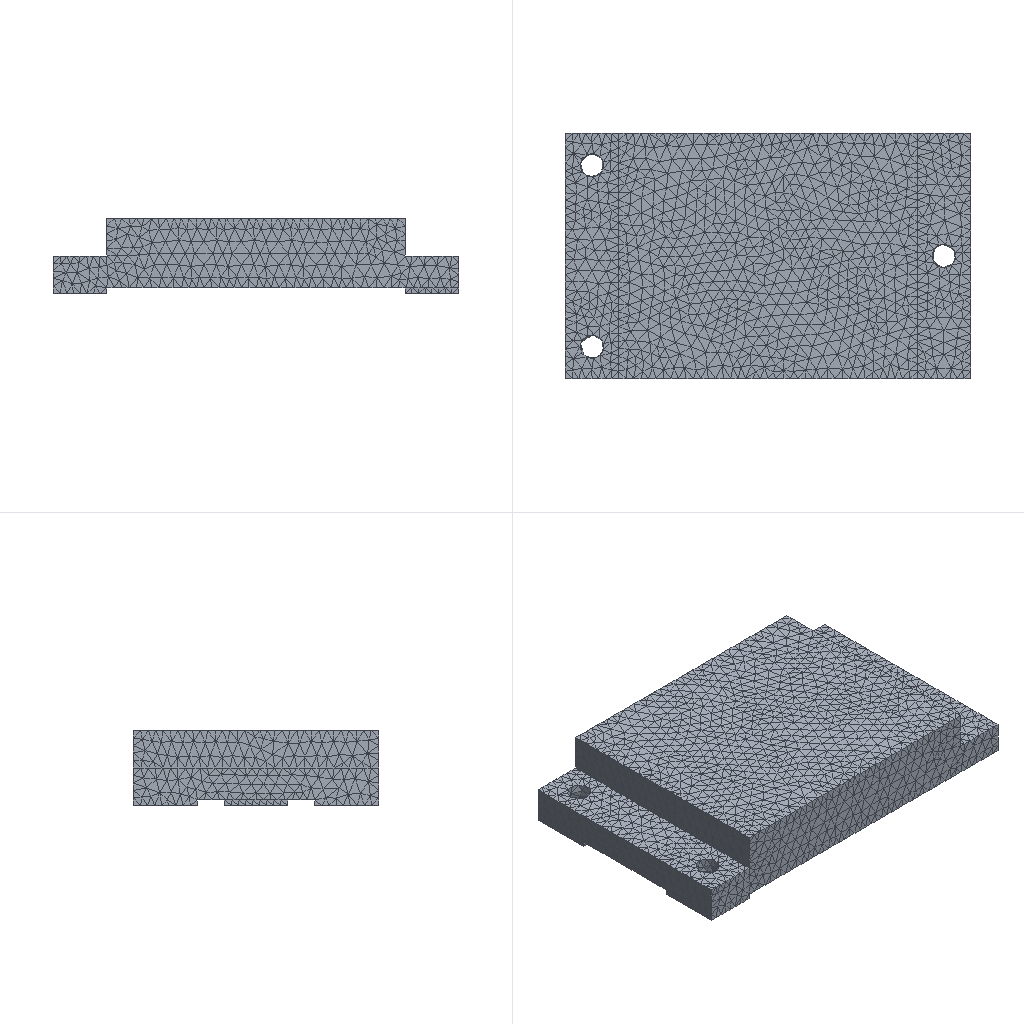Simulation study | ansys workbench
Set-up summary:
category,name,step,type,value,unit,region
solver,ansys_workbench
units,SI m-kg-s (Pa),,stated,"/units,MKS"
analysis,LS1,,static
load_step,LS1,LS1,static,nsubst=1; time=1
mesh,nodes,,,33082
mesh,elements,,,20941
element_type,SOLID187,,,19645
element_type,CONTA174,,,1296
material,Structural Steel,,E,2e+11,Pa
material,Structural Steel,,nu,0.3
material,Structural Steel,,density,7850,kg m^-3
material,Structural Steel,,conductivity,60.5,W m^-1 C^-1
material,Structural Steel,,specific_heat,434,J kg^-1 C^-1
material,Structural Steel,,cte,1.2e-05,C^-1
material,Structural Steel,,permeability,10000
material,Structural Steel,,resistivity,1.7e-07,kg m^3 A^-2 s^-3
load,,LS1,moment,"1500 [dir=(0, 0, 1) n=3]",,all
bc,Fixed Supports,model,fixed,[dofs=ALL],,_FIXEDSU
contact,contact 1,,bonded (always),element=CONTA174
named_set,_FIXEDSU,,node,597
Ansys APDL input file, long lists of numbers shortened:
/batch
/config,noeldb,1     ! force off writing results to database
*get,_wallstrt,active,,time,wall
! ANSYS input file written by Workbench version 2024 R1
! File used for geometry attach:
/title,wbnew--____ (A5)
! ****** Begin Custom Load Command Snippet ******
/COM, ACT Extensions:
/COM,     LSDYNA, 2024.1
/COM,/COM,     ANSYSMotion, 2024.1
/COM,
! ****** End   Custom Load Command Snippet ******
*DIM,_wb_ProjectScratch_dir,string,248
_wb_ProjectScratch_dir(1) = ''
*DIM,_wb_SolverFiles_dir,string,248
_wb_SolverFiles_dir(1) = ''
*DIM,_wb_userfiles_dir,string,248
_wb_userfiles_dir(1) = ''
/com,--- Data in consistent MKS units. See Solving Units in the help system for more information.
/units,MKS
/nopr
/wb,file,start              !  signify a WB generated input file
/prep7
! Turn off shape checking because checks already performed inside WB mesher.
! See help system for more information.
SHPP,OFF,,NOWARN
/nolist
etcon,set             ! allow ANSYS to choose best KEYOP's for 180x elements, resets any applicable keyopt to MAPDL defaults
/com,*********** Nodes for the whole assembly ***********
nblock,3,,36389
(1i9,3e20.9e3)
        1     7.600000000E-02     0.000000000E+00     1.000000000E-03
! (33080 more lines like these left out)
-1
/com,*********** Nodes for all Remote Points ***********
nblock,3
(1i9,3e20.9e3)
    33082     3.800000000E-02     2.300000000E-02     1.400000000E-02
-1
/wb,elem,start            !  set before creation of elements
/com,*********** Elements for Body 1 "__ - Camera Link" ***********
et,1,187
eblock,19,solid,,19645
(19i9)
        1        1        1        1        0        0        0        0       10        0        1     4123     5058     4344     5054    30312    31437    30307    30310
! (39289 more lines like these left out)
-1
/wb,elem,end               !  done creating elements
/com,*********** Send User Defined Coordinate System(s) ***********
csys,0
toffst,273.15,  ! Temperature offset from absolute zero
/com,*********** Set Reference Temperature ***********
tref,22.
/wb,mat,start              !  starting to send materials
/com,*********** Send Materials ***********
Temperature = 'TEMP' ! Temperature
MP,DENS,1,7850,	! kg m^-3
MP,ALPX,1,1.2e-05,	! C^-1
MP,C,1,434,	! J kg^-1 C^-1
MP,KXX,1,60.5,	! W m^-1 C^-1
MP,RSVX,1,1.7e-07,	! kg m^3 A^-2 s^-3
MP,EX,1,200000000000,	! Pa
MP,NUXY,1,0.3,
MP,MURX,1,10000,
/wb,mat,end                !  done sending materials
!************************* Model Summary ********************
!åºåº§ - Camera Link,	ç»æé¢,	matid,	1
!************************* End Model Summary ********************
! get the diagonal of the bounding box. Needed later for other things
*get,_xmin,node,,mnloc,x
*get,_ymin,node,,mnloc,y
*get,_zmin,node,,mnloc,z
*get,_xmax,node,,mxloc,x
*get,_ymax,node,,mxloc,y
*get,_zmax,node,,mxloc,z
_ASMDIAG=(_xmax-_xmin)*(_xmax-_xmin)+(_ymax-_ymin)*(_ymax-_ymin)+(_zmax-_zmin)*(_zmax-_zmin)
_ASMDIAG=SQRT(_ASMDIAG)
/wb,contact,start          !  starting to send contact
/wb,contact,end            !  done creating contacts
/golist
/wb,load,start             !  starting to send loads
/com,*********** Fixed Supports ***********
CMBLOCK,_FIXEDSU,NODE,      597
(8i10)
       120       125       126       127       128       129       130       131
! (74 more lines like these left out)
cmsel,s,_FIXEDSU
d,all,all
nsel,all
/com,*********** Create Remote Point "ÄÚ²¿Ô¶³Ìµã" ***********
! -------- Remote Point Used by "Á¦¾Ø" --------
*set,tid,3
*set,cid,2
et,cid,174
et,tid,170
keyo,tid,2,1               ! Don't fix the pilot node
keyo,tid,4,111111
keyo,cid,12,5              ! Bonded Contact
keyo,cid,4,1               ! Deformable RBE3 style load
keyo,cid,2,2               ! MPC style contact
eblock,10,,,1296
(15i9)
    26283        2        2        2        0     2862     3111     3238     3238    22444    23983     3238    22446
! (1295 more lines like these left out)
-1
*set,_npilot,33082
_npilot30=_npilot
type,tid
mat ,cid
real,cid
tshape,pilo
en,27579,_npilot
tshape
/com,*********** Construct Moment Using Remote Attachment ***********
/gst,on,on
fini
*get,_numnode,node,0,count
*get,_numelem,elem,0,count
*get, _MAXELEMNUM, elem, 0, NUM, MAX
*get, _MAXNODENUM, node, 0, NUM, MAX
*get, _MAXELEMTYPE, etyp, 0, NUM, MAX
*get, _MAXREALCONST, rcon, 0, NUM, MAX
/go
/wb,load,end               !  done creating loads
/com,--- Number of total nodes = %_numnode%
/com,--- Number of contact elements = 1296
/com,--- Number of spring elements = 0
/com,--- Number of bearing elements = 0
/com,--- Number of solid elements = 19645
/com,--- Number of condensed parts = 0
/com,--- Number of total elements = %_numelem%
*get,_wallbsol,active,,time,wall
/com,****************************************************************************
/com,*************************    SOLUTION       ********************************
/com,****************************************************************************
/solu
antype,0                   ! static analysis
_thickRatio=  1     ! Ratio of thick parts in the model
eqsl,pcg,1e-8,,,,,,1
cntr,print,1               ! print out contact info and also make no initial contact an error
cncheck,dmp		!	Enable program controlled contact splitting for distributed memory parallel run
dmpoption,emat,no             ! Don't combine emat file for DANSYS
dmpoption,esav,no             ! Don't combine esav file for DANSYS
nldiag,cont,iter           ! print out contact info each equilibrium iteration
rescontrol,,none                 ! Do not keep any restart files
/com,****************************************************
/com,******************* SOLVE FOR LS 1 OF 1 ****************
nsel,s,node,,33082
f,all,mx,0.
f,all,my,0.
f,all,mz,1500.
nsel,all
/nopr
/gopr
nsub,1,1,1
time,1.
outres,erase
outres,all,none
outres,nsol,all,
outres,rsol,all
outres,eangl,all
outres,etmp,all
outres,veng,all
outres,strs,all,
outres,epel,all,
outres,eppl,all,
outres,cont,all,
! *********** WB SOLVE COMMAND ***********
! check interactive state
*get,ANSINTER_,active,,int
*if,ANSINTER_,ne,0,then
/eof
*endif
solve
/com *************** Write FE CONNECTORS *********
CEWRITE,file,ce,,INTE
/com,****************************************************
/com,*************** FINISHED SOLVE FOR LS 1 *************
*get,_wallasol,active,,time,wall
/nopr
*get,_numnode,node,0,count
*get,_numelem,elem,0,count
*get, _MAXELEMNUM, elem, 0, NUM, MAX
*get, _MAXNODENUM, node, 0, NUM, MAX,,,INTERNAL
*get, _MAXELEMTYPE, etyp, 0, NUM, MAX
*get, _MAXREALCONST, rcon, 0, NUM, MAX
*get,_NSOLTHREADS,active,0,ntfs
*get,_NSOLPROCESSES,active,0,npfs
/gopr
*get,_PCGITER,active,,solu,cgiter
/post1
xmlo,ENCODING,ISO-8859-1
xmlo,parm
/xml,parm,xml
fini
/gopr
*get,_walldone,active,,time,wall
_preptime=(_wallbsol-_wallstrt)*3600
_solvtime=(_wallasol-_wallbsol)*3600
_posttime=(_walldone-_wallasol)*3600
_totaltim=(_walldone-_wallstrt)*3600
*get,_dlbratio,active,0,solu,dlbr
*get,_combtime,active,0,solu,comb
*get,_ssmode,active,0,solu,ssmm
*get,_ndofs,active,0,solu,ndof
*get,_sol_end_time,active,0,set,time
*if,_sol_end_time,eq,1.,then
/fclean				!clean distributed files
*endif
/com,--- Total number of nodes = %_numnode%
/com,--- Total number of elements = %_numelem%
/com,--- Element load balance ratio = %_dlbratio%
/com,--- Time to combine distributed files = %_combtime%
/com,--- Sparse memory mode = %_ssmode%
/com,--- Number of DOF = %_ndofs%
/wb,file,end               ! done with WB generated input
Results summary:
result,analyses[0].index,,,1
result,analyses[0].system,,,SYS
result,analyses[0].deck,,,deck.dat
result,analyses[0].solve_status,,,completed
result,analyses[0].analysis_type,,,static
result,analyses[0].physics,,,mechanical
result,analyses[0].unit_system,,,"MKS: m, kg, N, s, V, A, degC"
result,analyses[0].n_sets,,,1
result,analyses[0].load_steps[0].set,set=1,,1
result,analyses[0].load_steps[0].time_or_freq,set=1,,1
result,analyses[0].load_steps[0].max_displacement_magnitude,set=1,,8.3049e-05
result,analyses[0].load_steps[0].max_von_mises_nodal,set=1,,1.44359e+09
result,analyses[0].load_steps[0].reaction_force_sum_xyz[1],set=1,,1.39873e-05
result,analyses[0].load_steps[0].reaction_force_sum_xyz[2],set=1,,1.31882e-05
result,analyses[0].load_steps[0].reaction_force_sum_xyz[3],set=1,,-4.46866e-06
result,geometry_export[0][0],,,.step
result,geometry_export[0][1],,,ok
result,geometry_export[0][2],,,1